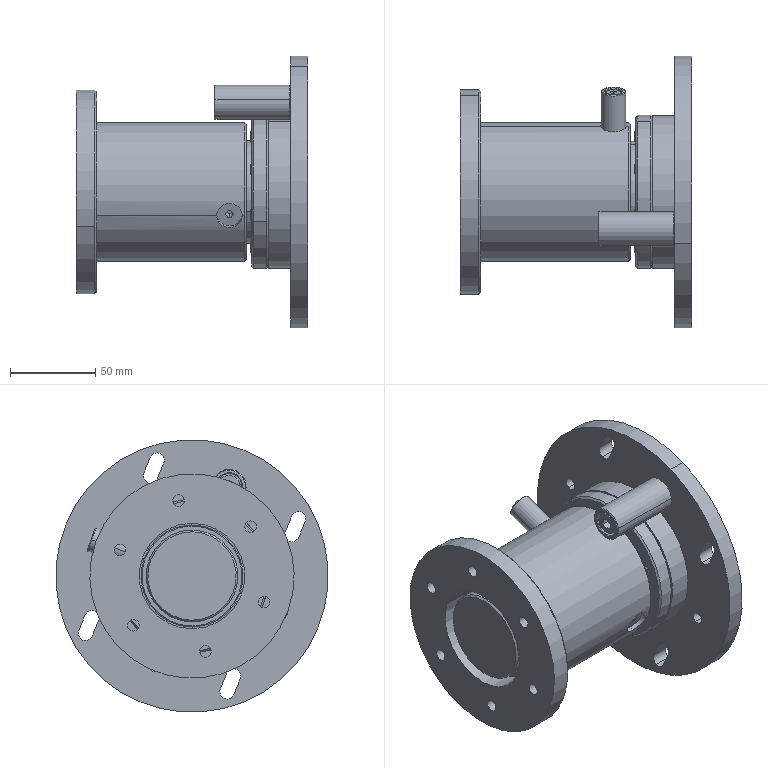Part | SolidWorks | features ReferencePattern 7, LocalCirPattern 1 | 23 solids | 936 faces | box 136 x 160 x 160 mm | volume 819562 mm3 | cylinder 251 | plane 245 | sphere 186 | torus 168 | cone 86 | commonest cylinder face diameters 6.8 x36 15 x22 8 x18 9 x18 13 x18 40 x13